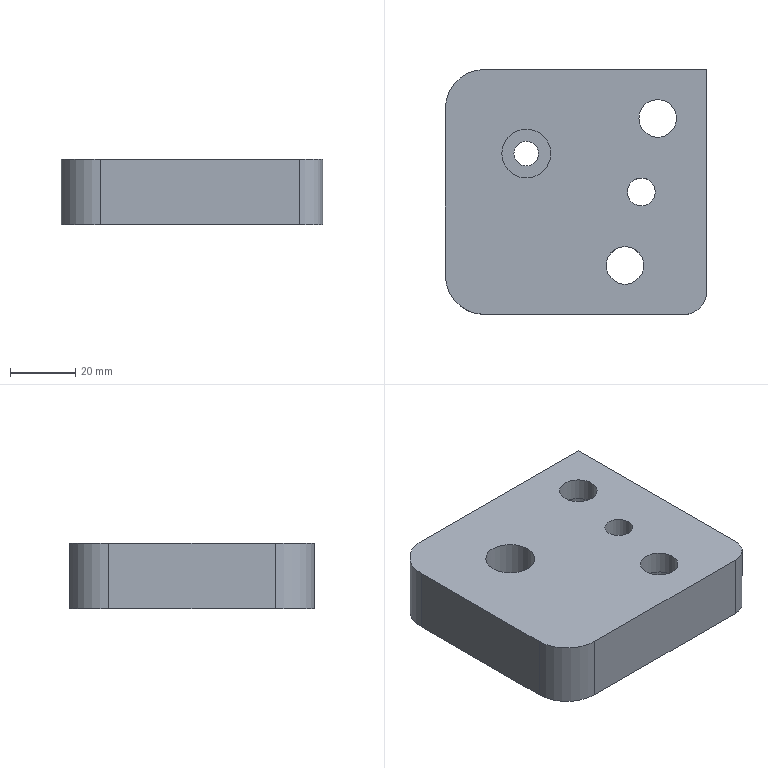Part | STEP file | lll_id94_x_t | 1 solid | 19 faces | box 80 x 75 x 20 mm | volume 106595 mm3 | cylinder 10 | plane 9 | commonest cylinder face diameters 11.509 x2 18.008 x2 24 x2 7.56 x1 8.505 x1 14 x1
STEP:
#1=CARTESIAN_POINT('',(786.993,-30.,2.5));
#2=VERTEX_POINT('',#1);
#3=CARTESIAN_POINT('',(790.773,-30.,2.5));
#4=DIRECTION('',(0.,0.,1.));
#5=DIRECTION('',(-1.,0.,0.));
#6=AXIS2_PLACEMENT_3D('',#3,#4,#5);
#7=CIRCLE('',#6,3.78);
#8=EDGE_CURVE('',#2,#2,#7,.T.);
#9=ORIENTED_EDGE('',*,*,#8,.T.);
#10=EDGE_LOOP('',(#9));
#11=FACE_BOUND('',#10,.T.);
#12=CARTESIAN_POINT('',(840.004,-19.25,2.5));
#13=VERTEX_POINT('',#12);
#14=CARTESIAN_POINT('',(831.,-19.25,2.5));
#15=DIRECTION('',(0.,0.,-1.));
#16=DIRECTION('',(1.,0.,0.));
#17=AXIS2_PLACEMENT_3D('',#14,#15,#16);
#18=CIRCLE('',#17,9.004);
#19=EDGE_CURVE('',#13,#13,#18,.T.);
#20=ORIENTED_EDGE('',*,*,#19,.F.);
#21=EDGE_LOOP('',(#20));
#22=FACE_BOUND('',#21,.T.);
#23=CARTESIAN_POINT('',(830.252,-41.75,2.5));
#24=VERTEX_POINT('',#23);
#25=CARTESIAN_POINT('',(826.,-41.75,2.5));
#26=DIRECTION('',(0.,0.,1.));
#27=DIRECTION('',(1.,0.,0.));
#28=AXIS2_PLACEMENT_3D('',#25,#26,#27);
#29=CIRCLE('',#28,4.253);
#30=EDGE_CURVE('',#24,#24,#29,.T.);
#31=ORIENTED_EDGE('',*,*,#30,.T.);
#32=EDGE_LOOP('',(#31));
#33=FACE_BOUND('',#32,.T.);
#34=CARTESIAN_POINT('',(846.,-72.25,2.5));
#35=VERTEX_POINT('',#34);
#36=CARTESIAN_POINT('',(846.,-4.25,2.5));
#37=VERTEX_POINT('',#36);
#38=CARTESIAN_POINT('',(846.,-16.75,2.5));
#39=DIRECTION('',(0.,1.,0.));
#40=VECTOR('',#39,1.);
#41=LINE('',#38,#40);
#42=EDGE_CURVE('',#35,#37,#41,.T.);
#43=ORIENTED_EDGE('',*,*,#42,.F.);
#44=CARTESIAN_POINT('',(839.,-79.25,2.5));
#45=VERTEX_POINT('',#44);
#46=CARTESIAN_POINT('',(839.,-72.25,2.5));
#47=DIRECTION('',(0.,0.,-1.));
#48=DIRECTION('',(-1.,0.,0.));
#49=AXIS2_PLACEMENT_3D('',#46,#47,#48);
#50=CIRCLE('',#49,7.);
#51=EDGE_CURVE('',#35,#45,#50,.T.);
#52=ORIENTED_EDGE('',*,*,#51,.T.);
#53=CARTESIAN_POINT('',(778.,-79.25,2.5));
#54=VERTEX_POINT('',#53);
#55=CARTESIAN_POINT('',(881.,-79.25,2.5));
#56=DIRECTION('',(1.,0.,0.));
#57=VECTOR('',#56,1.);
#58=LINE('',#55,#57);
#59=EDGE_CURVE('',#54,#45,#58,.T.);
#60=ORIENTED_EDGE('',*,*,#59,.F.);
#61=CARTESIAN_POINT('',(766.,-67.25,2.5));
#62=VERTEX_POINT('',#61);
#63=CARTESIAN_POINT('',(778.,-67.25,2.5));
#64=DIRECTION('',(0.,0.,-1.));
#65=DIRECTION('',(-1.,0.,0.));
#66=AXIS2_PLACEMENT_3D('',#63,#64,#65);
#67=CIRCLE('',#66,12.);
#68=EDGE_CURVE('',#54,#62,#67,.T.);
#69=ORIENTED_EDGE('',*,*,#68,.T.);
#70=CARTESIAN_POINT('',(766.,-16.25,2.5));
#71=VERTEX_POINT('',#70);
#72=CARTESIAN_POINT('',(766.,-16.75,2.5));
#73=DIRECTION('',(0.,-1.,0.));
#74=VECTOR('',#73,1.);
#75=LINE('',#72,#74);
#76=EDGE_CURVE('',#71,#62,#75,.T.);
#77=ORIENTED_EDGE('',*,*,#76,.F.);
#78=CARTESIAN_POINT('',(778.,-4.25,2.5));
#79=VERTEX_POINT('',#78);
#80=CARTESIAN_POINT('',(778.,-16.25,2.5));
#81=DIRECTION('',(0.,0.,-1.));
#82=DIRECTION('',(-1.,0.,0.));
#83=AXIS2_PLACEMENT_3D('',#80,#81,#82);
#84=CIRCLE('',#83,12.);
#85=EDGE_CURVE('',#71,#79,#84,.T.);
#86=ORIENTED_EDGE('',*,*,#85,.T.);
#87=CARTESIAN_POINT('',(881.,-4.25,2.5));
#88=DIRECTION('',(-1.,0.,0.));
#89=VECTOR('',#88,1.);
#90=LINE('',#87,#89);
#91=EDGE_CURVE('',#37,#79,#90,.T.);
#92=ORIENTED_EDGE('',*,*,#91,.F.);
#93=EDGE_LOOP('',(#43,#52,#60,#69,#77,#86,#92));
#94=FACE_BOUND('',#93,.T.);
#95=CARTESIAN_POINT('',(830.004,-64.25,2.5));
#96=VERTEX_POINT('',#95);
#97=CARTESIAN_POINT('',(821.,-64.25,2.5));
#98=DIRECTION('',(0.,0.,1.));
#99=DIRECTION('',(1.,0.,0.));
#100=AXIS2_PLACEMENT_3D('',#97,#98,#99);
#101=CIRCLE('',#100,9.004);
#102=EDGE_CURVE('',#96,#96,#101,.T.);
#103=ORIENTED_EDGE('',*,*,#102,.T.);
#104=EDGE_LOOP('',(#103));
#105=FACE_BOUND('',#104,.T.);
#106=CARTESIAN_POINT('',(881.,-16.75,2.5));
#107=DIRECTION('',(0.,0.,-1.));
#108=DIRECTION('',(-1.,0.,0.));
#109=AXIS2_PLACEMENT_3D('',#106,#107,#108);
#110=PLANE('',#109);
#111=ADVANCED_FACE('',(#11,#22,#33,#94,#105),#110,.T.);
#112=CARTESIAN_POINT('',(798.273,-30.,22.5));
#113=VERTEX_POINT('',#112);
#114=CARTESIAN_POINT('',(790.773,-30.,22.5));
#115=DIRECTION('',(0.,0.,-1.));
#116=DIRECTION('',(1.,0.,0.));
#117=AXIS2_PLACEMENT_3D('',#114,#115,#116);
#118=CIRCLE('',#117,7.5);
#119=EDGE_CURVE('',#113,#113,#118,.T.);
#120=ORIENTED_EDGE('',*,*,#119,.T.);
#121=EDGE_LOOP('',(#120));
#122=FACE_BOUND('',#121,.T.);
#123=CARTESIAN_POINT('',(836.754,-19.25,22.5));
#124=VERTEX_POINT('',#123);
#125=CARTESIAN_POINT('',(831.,-19.25,22.5));
#126=DIRECTION('',(0.,0.,1.));
#127=DIRECTION('',(1.,0.,0.));
#128=AXIS2_PLACEMENT_3D('',#125,#126,#127);
#129=CIRCLE('',#128,5.755);
#130=EDGE_CURVE('',#124,#124,#129,.T.);
#131=ORIENTED_EDGE('',*,*,#130,.F.);
#132=EDGE_LOOP('',(#131));
#133=FACE_BOUND('',#132,.T.);
#134=CARTESIAN_POINT('',(839.,-79.25,22.5));
#135=VERTEX_POINT('',#134);
#136=CARTESIAN_POINT('',(778.,-79.25,22.5));
#137=VERTEX_POINT('',#136);
#138=CARTESIAN_POINT('',(881.,-79.25,22.5));
#139=DIRECTION('',(-1.,0.,0.));
#140=VECTOR('',#139,1.);
#141=LINE('',#138,#140);
#142=EDGE_CURVE('',#135,#137,#141,.T.);
#143=ORIENTED_EDGE('',*,*,#142,.F.);
#144=CARTESIAN_POINT('',(846.,-72.25,22.5));
#145=VERTEX_POINT('',#144);
#146=CARTESIAN_POINT('',(839.,-72.25,22.5));
#147=DIRECTION('',(0.,0.,1.));
#148=DIRECTION('',(1.,0.,0.));
#149=AXIS2_PLACEMENT_3D('',#146,#147,#148);
#150=CIRCLE('',#149,7.);
#151=EDGE_CURVE('',#135,#145,#150,.T.);
#152=ORIENTED_EDGE('',*,*,#151,.T.);
#153=CARTESIAN_POINT('',(846.,-4.25,22.5));
#154=VERTEX_POINT('',#153);
#155=CARTESIAN_POINT('',(846.,-16.75,22.5));
#156=DIRECTION('',(0.,-1.,0.));
#157=VECTOR('',#156,1.);
#158=LINE('',#155,#157);
#159=EDGE_CURVE('',#154,#145,#158,.T.);
#160=ORIENTED_EDGE('',*,*,#159,.F.);
#161=CARTESIAN_POINT('',(778.,-4.25,22.5));
#162=VERTEX_POINT('',#161);
#163=CARTESIAN_POINT('',(881.,-4.25,22.5));
#164=DIRECTION('',(1.,0.,0.));
#165=VECTOR('',#164,1.);
#166=LINE('',#163,#165);
#167=EDGE_CURVE('',#162,#154,#166,.T.);
#168=ORIENTED_EDGE('',*,*,#167,.F.);
#169=CARTESIAN_POINT('',(766.,-16.25,22.5));
#170=VERTEX_POINT('',#169);
#171=CARTESIAN_POINT('',(778.,-16.25,22.5));
#172=DIRECTION('',(0.,0.,1.));
#173=DIRECTION('',(1.,0.,0.));
#174=AXIS2_PLACEMENT_3D('',#171,#172,#173);
#175=CIRCLE('',#174,12.);
#176=EDGE_CURVE('',#162,#170,#175,.T.);
#177=ORIENTED_EDGE('',*,*,#176,.T.);
#178=CARTESIAN_POINT('',(766.,-67.25,22.5));
#179=VERTEX_POINT('',#178);
#180=CARTESIAN_POINT('',(766.,-16.75,22.5));
#181=DIRECTION('',(0.,-1.,0.));
#182=VECTOR('',#181,1.);
#183=LINE('',#180,#182);
#184=EDGE_CURVE('',#170,#179,#183,.T.);
#185=ORIENTED_EDGE('',*,*,#184,.T.);
#186=CARTESIAN_POINT('',(778.,-67.25,22.5));
#187=DIRECTION('',(0.,0.,1.));
#188=DIRECTION('',(1.,0.,0.));
#189=AXIS2_PLACEMENT_3D('',#186,#187,#188);
#190=CIRCLE('',#189,12.);
#191=EDGE_CURVE('',#179,#137,#190,.T.);
#192=ORIENTED_EDGE('',*,*,#191,.T.);
#193=EDGE_LOOP('',(#143,#152,#160,#168,#177,#185,#192));
#194=FACE_BOUND('',#193,.T.);
#195=CARTESIAN_POINT('',(830.252,-41.75,22.5));
#196=VERTEX_POINT('',#195);
#197=CARTESIAN_POINT('',(826.,-41.75,22.5));
#198=DIRECTION('',(0.,0.,1.));
#199=DIRECTION('',(1.,0.,0.));
#200=AXIS2_PLACEMENT_3D('',#197,#198,#199);
#201=CIRCLE('',#200,4.253);
#202=EDGE_CURVE('',#196,#196,#201,.T.);
#203=ORIENTED_EDGE('',*,*,#202,.F.);
#204=EDGE_LOOP('',(#203));
#205=FACE_BOUND('',#204,.T.);
#206=CARTESIAN_POINT('',(826.754,-64.25,22.5));
#207=VERTEX_POINT('',#206);
#208=CARTESIAN_POINT('',(821.,-64.25,22.5));
#209=DIRECTION('',(0.,0.,-1.));
#210=DIRECTION('',(1.,0.,0.));
#211=AXIS2_PLACEMENT_3D('',#208,#209,#210);
#212=CIRCLE('',#211,5.755);
#213=EDGE_CURVE('',#207,#207,#212,.T.);
#214=ORIENTED_EDGE('',*,*,#213,.T.);
#215=EDGE_LOOP('',(#214));
#216=FACE_BOUND('',#215,.T.);
#217=CARTESIAN_POINT('',(881.,-16.75,22.5));
#218=DIRECTION('',(0.,0.,1.));
#219=DIRECTION('',(1.,0.,0.));
#220=AXIS2_PLACEMENT_3D('',#217,#218,#219);
#221=PLANE('',#220);
#222=ADVANCED_FACE('',(#122,#133,#194,#205,#216),#221,.T.);
#223=ORIENTED_EDGE('',*,*,#59,.T.);
#224=CARTESIAN_POINT('',(839.,-79.25,2.5));
#225=DIRECTION('',(0.,0.,1.));
#226=VECTOR('',#225,1.);
#227=LINE('',#224,#226);
#228=EDGE_CURVE('',#45,#135,#227,.T.);
#229=ORIENTED_EDGE('',*,*,#228,.T.);
#230=ORIENTED_EDGE('',*,*,#142,.T.);
#231=CARTESIAN_POINT('',(778.,-79.25,2.5));
#232=DIRECTION('',(0.,0.,-1.));
#233=VECTOR('',#232,1.);
#234=LINE('',#231,#233);
#235=EDGE_CURVE('',#137,#54,#234,.T.);
#236=ORIENTED_EDGE('',*,*,#235,.T.);
#237=EDGE_LOOP('',(#223,#229,#230,#236));
#238=FACE_OUTER_BOUND('',#237,.T.);
#239=CARTESIAN_POINT('',(881.,-79.25,2.5));
#240=DIRECTION('',(0.,-1.,0.));
#241=DIRECTION('',(0.,0.,-1.));
#242=AXIS2_PLACEMENT_3D('',#239,#240,#241);
#243=PLANE('',#242);
#244=ADVANCED_FACE('',(#238),#243,.T.);
#245=ORIENTED_EDGE('',*,*,#184,.F.);
#246=CARTESIAN_POINT('',(766.,-16.25,12.5));
#247=DIRECTION('',(0.,0.,-1.));
#248=VECTOR('',#247,1.);
#249=LINE('',#246,#248);
#250=EDGE_CURVE('',#170,#71,#249,.T.);
#251=ORIENTED_EDGE('',*,*,#250,.T.);
#252=ORIENTED_EDGE('',*,*,#76,.T.);
#253=CARTESIAN_POINT('',(766.,-67.25,12.5));
#254=DIRECTION('',(0.,0.,1.));
#255=VECTOR('',#254,1.);
#256=LINE('',#253,#255);
#257=EDGE_CURVE('',#62,#179,#256,.T.);
#258=ORIENTED_EDGE('',*,*,#257,.T.);
#259=EDGE_LOOP('',(#245,#251,#252,#258));
#260=FACE_OUTER_BOUND('',#259,.T.);
#261=CARTESIAN_POINT('',(766.,-16.75,12.5));
#262=DIRECTION('',(-1.,0.,0.));
#263=DIRECTION('',(0.,0.,1.));
#264=AXIS2_PLACEMENT_3D('',#261,#262,#263);
#265=PLANE('',#264);
#266=ADVANCED_FACE('',(#260),#265,.T.);
#267=ORIENTED_EDGE('',*,*,#167,.T.);
#268=CARTESIAN_POINT('',(846.,-4.25,2.5));
#269=DIRECTION('',(0.,0.,1.));
#270=VECTOR('',#269,1.);
#271=LINE('',#268,#270);
#272=EDGE_CURVE('',#37,#154,#271,.T.);
#273=ORIENTED_EDGE('',*,*,#272,.F.);
#274=ORIENTED_EDGE('',*,*,#91,.T.);
#275=CARTESIAN_POINT('',(778.,-4.25,2.5));
#276=DIRECTION('',(0.,0.,1.));
#277=VECTOR('',#276,1.);
#278=LINE('',#275,#277);
#279=EDGE_CURVE('',#79,#162,#278,.T.);
#280=ORIENTED_EDGE('',*,*,#279,.T.);
#281=EDGE_LOOP('',(#267,#273,#274,#280));
#282=FACE_OUTER_BOUND('',#281,.T.);
#283=CARTESIAN_POINT('',(881.,-4.25,2.5));
#284=DIRECTION('',(0.,1.,0.));
#285=DIRECTION('',(0.,0.,1.));
#286=AXIS2_PLACEMENT_3D('',#283,#284,#285);
#287=PLANE('',#286);
#288=ADVANCED_FACE('',(#282),#287,.T.);
#289=ORIENTED_EDGE('',*,*,#176,.F.);
#290=ORIENTED_EDGE('',*,*,#279,.F.);
#291=ORIENTED_EDGE('',*,*,#85,.F.);
#292=ORIENTED_EDGE('',*,*,#250,.F.);
#293=EDGE_LOOP('',(#289,#290,#291,#292));
#294=FACE_OUTER_BOUND('',#293,.T.);
#295=CARTESIAN_POINT('',(778.,-16.25,12.5));
#296=DIRECTION('',(0.,0.,-1.));
#297=DIRECTION('',(-1.,0.,0.));
#298=AXIS2_PLACEMENT_3D('',#295,#296,#297);
#299=CYLINDRICAL_SURFACE('',#298,12.);
#300=ADVANCED_FACE('',(#294),#299,.T.);
#301=ORIENTED_EDGE('',*,*,#191,.F.);
#302=ORIENTED_EDGE('',*,*,#257,.F.);
#303=ORIENTED_EDGE('',*,*,#68,.F.);
#304=ORIENTED_EDGE('',*,*,#235,.F.);
#305=EDGE_LOOP('',(#301,#302,#303,#304));
#306=FACE_OUTER_BOUND('',#305,.T.);
#307=CARTESIAN_POINT('',(778.,-67.25,2.5));
#308=DIRECTION('',(0.,0.,-1.));
#309=DIRECTION('',(-1.,0.,0.));
#310=AXIS2_PLACEMENT_3D('',#307,#308,#309);
#311=CYLINDRICAL_SURFACE('',#310,12.);
#312=ADVANCED_FACE('',(#306),#311,.T.);
#313=ORIENTED_EDGE('',*,*,#159,.T.);
#314=CARTESIAN_POINT('',(846.,-72.25,2.5));
#315=DIRECTION('',(0.,0.,-1.));
#316=VECTOR('',#315,1.);
#317=LINE('',#314,#316);
#318=EDGE_CURVE('',#145,#35,#317,.T.);
#319=ORIENTED_EDGE('',*,*,#318,.T.);
#320=ORIENTED_EDGE('',*,*,#42,.T.);
#321=ORIENTED_EDGE('',*,*,#272,.T.);
#322=EDGE_LOOP('',(#313,#319,#320,#321));
#323=FACE_OUTER_BOUND('',#322,.T.);
#324=CARTESIAN_POINT('',(846.,17.25,12.5));
#325=DIRECTION('',(-1.,0.,0.));
#326=DIRECTION('',(0.,0.,1.));
#327=AXIS2_PLACEMENT_3D('',#324,#325,#326);
#328=PLANE('',#327);
#329=ADVANCED_FACE('',(#323),#328,.F.);
#330=ORIENTED_EDGE('',*,*,#202,.T.);
#331=EDGE_LOOP('',(#330));
#332=FACE_BOUND('',#331,.T.);
#333=ORIENTED_EDGE('',*,*,#30,.F.);
#334=EDGE_LOOP('',(#333));
#335=FACE_BOUND('',#334,.T.);
#336=CARTESIAN_POINT('',(826.,-41.75,2.5));
#337=DIRECTION('',(0.,0.,1.));
#338=DIRECTION('',(1.,0.,0.));
#339=AXIS2_PLACEMENT_3D('',#336,#337,#338);
#340=CYLINDRICAL_SURFACE('',#339,4.253);
#341=ADVANCED_FACE('',(#332,#335),#340,.F.);
#342=ORIENTED_EDGE('',*,*,#151,.F.);
#343=ORIENTED_EDGE('',*,*,#228,.F.);
#344=ORIENTED_EDGE('',*,*,#51,.F.);
#345=ORIENTED_EDGE('',*,*,#318,.F.);
#346=EDGE_LOOP('',(#342,#343,#344,#345));
#347=FACE_OUTER_BOUND('',#346,.T.);
#348=CARTESIAN_POINT('',(839.,-72.25,2.5));
#349=DIRECTION('',(0.,0.,-1.));
#350=DIRECTION('',(-1.,0.,0.));
#351=AXIS2_PLACEMENT_3D('',#348,#349,#350);
#352=CYLINDRICAL_SURFACE('',#351,7.);
#353=ADVANCED_FACE('',(#347),#352,.T.);
#354=CARTESIAN_POINT('',(826.754,-64.25,15.5));
#355=VERTEX_POINT('',#354);
#356=CARTESIAN_POINT('',(821.,-64.25,15.5));
#357=DIRECTION('',(0.,0.,1.));
#358=DIRECTION('',(1.,0.,0.));
#359=AXIS2_PLACEMENT_3D('',#356,#357,#358);
#360=CIRCLE('',#359,5.755);
#361=EDGE_CURVE('',#355,#355,#360,.T.);
#362=ORIENTED_EDGE('',*,*,#361,.F.);
#363=EDGE_LOOP('',(#362));
#364=FACE_BOUND('',#363,.T.);
#365=ORIENTED_EDGE('',*,*,#213,.F.);
#366=EDGE_LOOP('',(#365));
#367=FACE_BOUND('',#366,.T.);
#368=CARTESIAN_POINT('',(821.,-64.25,2.5));
#369=DIRECTION('',(0.,0.,1.));
#370=DIRECTION('',(1.,0.,0.));
#371=AXIS2_PLACEMENT_3D('',#368,#369,#370);
#372=CYLINDRICAL_SURFACE('',#371,5.755);
#373=ADVANCED_FACE('',(#364,#367),#372,.F.);
#374=ORIENTED_EDGE('',*,*,#361,.T.);
#375=EDGE_LOOP('',(#374));
#376=FACE_BOUND('',#375,.T.);
#377=CARTESIAN_POINT('',(830.004,-64.25,15.5));
#378=VERTEX_POINT('',#377);
#379=CARTESIAN_POINT('',(821.,-64.25,15.5));
#380=DIRECTION('',(0.,0.,1.));
#381=DIRECTION('',(1.,0.,0.));
#382=AXIS2_PLACEMENT_3D('',#379,#380,#381);
#383=CIRCLE('',#382,9.004);
#384=EDGE_CURVE('',#378,#378,#383,.T.);
#385=ORIENTED_EDGE('',*,*,#384,.F.);
#386=EDGE_LOOP('',(#385));
#387=FACE_BOUND('',#386,.T.);
#388=CARTESIAN_POINT('',(821.,-64.25,15.5));
#389=DIRECTION('',(0.,0.,1.));
#390=DIRECTION('',(1.,0.,0.));
#391=AXIS2_PLACEMENT_3D('',#388,#389,#390);
#392=PLANE('',#391);
#393=ADVANCED_FACE('',(#376,#387),#392,.F.);
#394=ORIENTED_EDGE('',*,*,#384,.T.);
#395=EDGE_LOOP('',(#394));
#396=FACE_BOUND('',#395,.T.);
#397=ORIENTED_EDGE('',*,*,#102,.F.);
#398=EDGE_LOOP('',(#397));
#399=FACE_BOUND('',#398,.T.);
#400=CARTESIAN_POINT('',(821.,-64.25,2.5));
#401=DIRECTION('',(0.,0.,1.));
#402=DIRECTION('',(1.,0.,0.));
#403=AXIS2_PLACEMENT_3D('',#400,#401,#402);
#404=CYLINDRICAL_SURFACE('',#403,9.004);
#405=ADVANCED_FACE('',(#396,#399),#404,.F.);
#406=CARTESIAN_POINT('',(836.754,-19.25,15.5));
#407=VERTEX_POINT('',#406);
#408=CARTESIAN_POINT('',(831.,-19.25,15.5));
#409=DIRECTION('',(0.,0.,-1.));
#410=DIRECTION('',(1.,0.,0.));
#411=AXIS2_PLACEMENT_3D('',#408,#409,#410);
#412=CIRCLE('',#411,5.755);
#413=EDGE_CURVE('',#407,#407,#412,.T.);
#414=ORIENTED_EDGE('',*,*,#413,.T.);
#415=EDGE_LOOP('',(#414));
#416=FACE_BOUND('',#415,.T.);
#417=ORIENTED_EDGE('',*,*,#130,.T.);
#418=EDGE_LOOP('',(#417));
#419=FACE_BOUND('',#418,.T.);
#420=CARTESIAN_POINT('',(831.,-19.25,2.5));
#421=DIRECTION('',(0.,0.,1.));
#422=DIRECTION('',(1.,0.,0.));
#423=AXIS2_PLACEMENT_3D('',#420,#421,#422);
#424=CYLINDRICAL_SURFACE('',#423,5.755);
#425=ADVANCED_FACE('',(#416,#419),#424,.F.);
#426=ORIENTED_EDGE('',*,*,#413,.F.);
#427=EDGE_LOOP('',(#426));
#428=FACE_BOUND('',#427,.T.);
#429=CARTESIAN_POINT('',(840.004,-19.25,15.5));
#430=VERTEX_POINT('',#429);
#431=CARTESIAN_POINT('',(831.,-19.25,15.5));
#432=DIRECTION('',(0.,0.,-1.));
#433=DIRECTION('',(1.,0.,0.));
#434=AXIS2_PLACEMENT_3D('',#431,#432,#433);
#435=CIRCLE('',#434,9.004);
#436=EDGE_CURVE('',#430,#430,#435,.T.);
#437=ORIENTED_EDGE('',*,*,#436,.T.);
#438=EDGE_LOOP('',(#437));
#439=FACE_BOUND('',#438,.T.);
#440=CARTESIAN_POINT('',(831.,-19.25,15.5));
#441=DIRECTION('',(0.,0.,1.));
#442=DIRECTION('',(1.,0.,0.));
#443=AXIS2_PLACEMENT_3D('',#440,#441,#442);
#444=PLANE('',#443);
#445=ADVANCED_FACE('',(#428,#439),#444,.F.);
#446=ORIENTED_EDGE('',*,*,#436,.F.);
#447=EDGE_LOOP('',(#446));
#448=FACE_BOUND('',#447,.T.);
#449=ORIENTED_EDGE('',*,*,#19,.T.);
#450=EDGE_LOOP('',(#449));
#451=FACE_BOUND('',#450,.T.);
#452=CARTESIAN_POINT('',(831.,-19.25,2.5));
#453=DIRECTION('',(0.,0.,1.));
#454=DIRECTION('',(1.,0.,0.));
#455=AXIS2_PLACEMENT_3D('',#452,#453,#454);
#456=CYLINDRICAL_SURFACE('',#455,9.004);
#457=ADVANCED_FACE('',(#448,#451),#456,.F.);
#458=ORIENTED_EDGE('',*,*,#8,.F.);
#459=EDGE_LOOP('',(#458));
#460=FACE_BOUND('',#459,.T.);
#461=CARTESIAN_POINT('',(786.993,-30.,8.5));
#462=VERTEX_POINT('',#461);
#463=CARTESIAN_POINT('',(790.773,-30.,8.5));
#464=DIRECTION('',(0.,0.,-1.));
#465=DIRECTION('',(-1.,0.,0.));
#466=AXIS2_PLACEMENT_3D('',#463,#464,#465);
#467=CIRCLE('',#466,3.78);
#468=EDGE_CURVE('',#462,#462,#467,.T.);
#469=ORIENTED_EDGE('',*,*,#468,.F.);
#470=EDGE_LOOP('',(#469));
#471=FACE_BOUND('',#470,.T.);
#472=CARTESIAN_POINT('',(790.773,-30.,12.5));
#473=DIRECTION('',(0.,0.,-1.));
#474=DIRECTION('',(-1.,0.,0.));
#475=AXIS2_PLACEMENT_3D('',#472,#473,#474);
#476=CYLINDRICAL_SURFACE('',#475,3.78);
#477=ADVANCED_FACE('',(#460,#471),#476,.F.);
#478=CARTESIAN_POINT('',(783.273,-30.,8.5));
#479=VERTEX_POINT('',#478);
#480=CARTESIAN_POINT('',(790.773,-30.,8.5));
#481=DIRECTION('',(0.,0.,-1.));
#482=DIRECTION('',(-1.,0.,0.));
#483=AXIS2_PLACEMENT_3D('',#480,#481,#482);
#484=CIRCLE('',#483,7.5);
#485=EDGE_CURVE('',#479,#479,#484,.T.);
#486=ORIENTED_EDGE('',*,*,#485,.T.);
#487=EDGE_LOOP('',(#486));
#488=FACE_BOUND('',#487,.T.);
#489=ORIENTED_EDGE('',*,*,#119,.F.);
#490=EDGE_LOOP('',(#489));
#491=FACE_BOUND('',#490,.T.);
#492=CARTESIAN_POINT('',(790.773,-30.,22.5));
#493=DIRECTION('',(0.,0.,-1.));
#494=DIRECTION('',(-1.,0.,0.));
#495=AXIS2_PLACEMENT_3D('',#492,#493,#494);
#496=CYLINDRICAL_SURFACE('',#495,7.5);
#497=ADVANCED_FACE('',(#488,#491),#496,.F.);
#498=ORIENTED_EDGE('',*,*,#468,.T.);
#499=EDGE_LOOP('',(#498));
#500=FACE_BOUND('',#499,.T.);
#501=ORIENTED_EDGE('',*,*,#485,.F.);
#502=EDGE_LOOP('',(#501));
#503=FACE_BOUND('',#502,.T.);
#504=CARTESIAN_POINT('',(790.773,-30.,8.5));
#505=DIRECTION('',(0.,0.,-1.));
#506=DIRECTION('',(-1.,0.,0.));
#507=AXIS2_PLACEMENT_3D('',#504,#505,#506);
#508=PLANE('',#507);
#509=ADVANCED_FACE('',(#500,#503),#508,.F.);
#510=CLOSED_SHELL('',(#111,#222,#244,#266,#288,#300,#312,#329,#341,#353,#373,#393,#405,#425,#445,#457,#477,#497,#509));
#511=MANIFOLD_SOLID_BREP('',#510);
#512=(LENGTH_UNIT()NAMED_UNIT(*)SI_UNIT(.MILLI.,.METRE.));
#513=UNCERTAINTY_MEASURE_WITH_UNIT(LENGTH_MEASURE(0.00002),#512,'','');
#514=(NAMED_UNIT(*)PLANE_ANGLE_UNIT()SI_UNIT($,.RADIAN.));
#515=PLANE_ANGLE_MEASURE_WITH_UNIT(PLANE_ANGLE_MEASURE(0.01745),#514);
#516=DIMENSIONAL_EXPONENTS(0.,0.,0.,0.,0.,0.,0.);
#517=(CONVERSION_BASED_UNIT('DEGREE',#515)NAMED_UNIT(#516)PLANE_ANGLE_UNIT());
#518=(NAMED_UNIT(*)SI_UNIT($,.STERADIAN.)SOLID_ANGLE_UNIT());
#519=(GEOMETRIC_REPRESENTATION_CONTEXT(3)GLOBAL_UNCERTAINTY_ASSIGNED_CONTEXT((#513))GLOBAL_UNIT_ASSIGNED_CONTEXT((#512,#517,#518))REPRESENTATION_CONTEXT('',''));
#520=ADVANCED_BREP_SHAPE_REPRESENTATION('',(#511),#519);